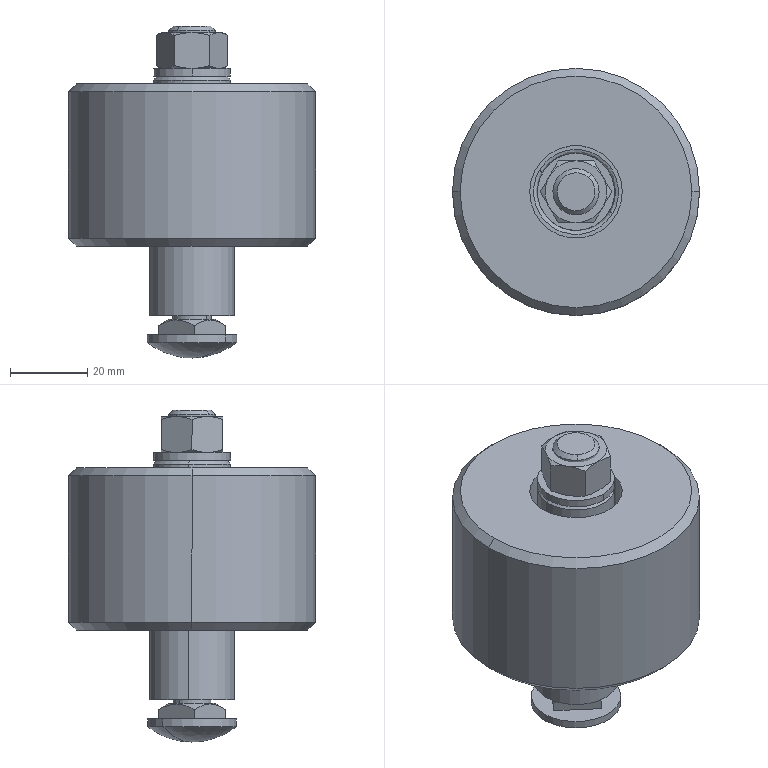Part | SolidWorks | features LayoutProfileFeature 1 | 5 solids | 177 faces | box 64 x 64 x 86 mm | volume 122485 mm3 | spline 58 | cylinder 56 | plane 35 | cone 28 | commonest cylinder face diameters 20 x8 28.802 x8 38.198 x8 47 x6 27.362 x4 39.638 x4